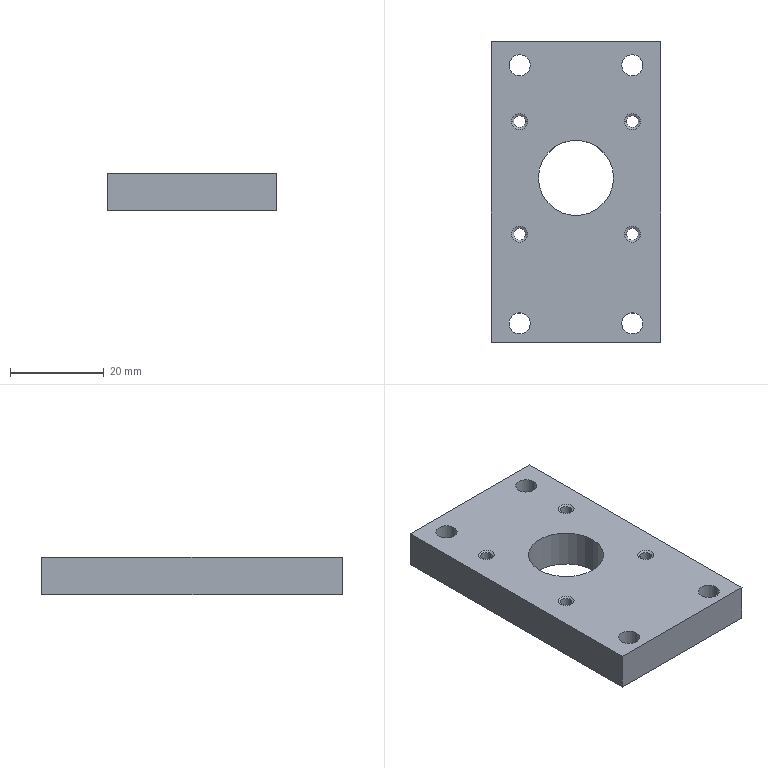Part | NX | 1 solid | 32 faces | box 36.002 x 64 x 8.011 mm | volume 16155 mm3 | cylinder 18 | cone 8 | plane 6 | commonest cylinder face diameters 2.5 x8 4.5 x8 16 x2
STEP:
#1=CARTESIAN_POINT('',(1234.583,117.5,67.602));
#2=VERTEX_POINT('',#1);
#3=CARTESIAN_POINT('',(1198.583,117.5,67.613));
#4=VERTEX_POINT('',#3);
#5=CARTESIAN_POINT('',(1211.755,117.5,67.609));
#6=DIRECTION('',(-1.,0.,0.0003046));
#7=VECTOR('',#6,1000.);
#8=LINE('',#5,#7);
#9=EDGE_CURVE('',#2,#4,#8,.T.);
#10=ORIENTED_EDGE('',*,*,#9,.F.);
#11=CARTESIAN_POINT('',(1234.585,117.5,75.602));
#12=VERTEX_POINT('',#11);
#13=CARTESIAN_POINT('',(1234.582,117.5,65.602));
#14=DIRECTION('',(0.0003046,0.,1.));
#15=VECTOR('',#14,1000.);
#16=LINE('',#13,#15);
#17=EDGE_CURVE('',#2,#12,#16,.T.);
#18=ORIENTED_EDGE('',*,*,#17,.T.);
#19=CARTESIAN_POINT('',(1198.585,117.5,75.613));
#20=VERTEX_POINT('',#19);
#21=CARTESIAN_POINT('',(1211.758,117.5,75.609));
#22=DIRECTION('',(-1.,0.,0.0003046));
#23=VECTOR('',#22,1000.);
#24=LINE('',#21,#23);
#25=EDGE_CURVE('',#12,#20,#24,.T.);
#26=ORIENTED_EDGE('',*,*,#25,.T.);
#27=CARTESIAN_POINT('',(1198.582,117.5,65.613));
#28=DIRECTION('',(-0.0003046,0.,-1.));
#29=VECTOR('',#28,1000.);
#30=LINE('',#27,#29);
#31=EDGE_CURVE('',#20,#4,#30,.T.);
#32=ORIENTED_EDGE('',*,*,#31,.T.);
#33=EDGE_LOOP('',(#10,#18,#26,#32));
#34=FACE_BOUND('',#33,.T.);
#35=CARTESIAN_POINT('',(1236.582,117.5,65.601));
#36=DIRECTION('',(0.,-1.,0.));
#37=DIRECTION('',(0.,0.,-1.));
#38=AXIS2_PLACEMENT_3D('',#35,#36,#37);
#39=PLANE('',#38);
#40=ADVANCED_FACE('',(#34),#39,.T.);
#41=CARTESIAN_POINT('',(1234.583,181.5,67.602));
#42=VERTEX_POINT('',#41);
#43=CARTESIAN_POINT('',(1234.583,131.898,67.602));
#44=DIRECTION('',(0.,-1.,0.));
#45=VECTOR('',#44,1000.);
#46=LINE('',#43,#45);
#47=EDGE_CURVE('',#42,#2,#46,.T.);
#48=ORIENTED_EDGE('',*,*,#47,.F.);
#49=CARTESIAN_POINT('',(1234.585,181.5,75.602));
#50=VERTEX_POINT('',#49);
#51=CARTESIAN_POINT('',(1234.582,181.5,65.602));
#52=DIRECTION('',(0.0003046,0.,1.));
#53=VECTOR('',#52,1000.);
#54=LINE('',#51,#53);
#55=EDGE_CURVE('',#42,#50,#54,.T.);
#56=ORIENTED_EDGE('',*,*,#55,.T.);
#57=CARTESIAN_POINT('',(1234.585,131.898,75.602));
#58=DIRECTION('',(0.,-1.,0.));
#59=VECTOR('',#58,1000.);
#60=LINE('',#57,#59);
#61=EDGE_CURVE('',#50,#12,#60,.T.);
#62=ORIENTED_EDGE('',*,*,#61,.T.);
#63=ORIENTED_EDGE('',*,*,#17,.F.);
#64=EDGE_LOOP('',(#48,#56,#62,#63));
#65=FACE_BOUND('',#64,.T.);
#66=CARTESIAN_POINT('',(1234.582,127.5,65.602));
#67=DIRECTION('',(1.,0.,-0.0003046));
#68=DIRECTION('',(0.,-1.,0.));
#69=AXIS2_PLACEMENT_3D('',#66,#67,#68);
#70=PLANE('',#69);
#71=ADVANCED_FACE('',(#65),#70,.T.);
#72=CARTESIAN_POINT('',(1198.583,181.5,67.613));
#73=VERTEX_POINT('',#72);
#74=CARTESIAN_POINT('',(1211.755,181.5,67.609));
#75=DIRECTION('',(1.,0.,-0.0003046));
#76=VECTOR('',#75,1000.);
#77=LINE('',#74,#76);
#78=EDGE_CURVE('',#73,#42,#77,.T.);
#79=ORIENTED_EDGE('',*,*,#78,.F.);
#80=CARTESIAN_POINT('',(1198.585,181.5,75.613));
#81=VERTEX_POINT('',#80);
#82=CARTESIAN_POINT('',(1198.582,181.5,65.613));
#83=DIRECTION('',(-0.0003046,0.,-1.));
#84=VECTOR('',#83,1000.);
#85=LINE('',#82,#84);
#86=EDGE_CURVE('',#81,#73,#85,.T.);
#87=ORIENTED_EDGE('',*,*,#86,.F.);
#88=CARTESIAN_POINT('',(1211.758,181.5,75.609));
#89=DIRECTION('',(1.,0.,-0.0003046));
#90=VECTOR('',#89,1000.);
#91=LINE('',#88,#90);
#92=EDGE_CURVE('',#81,#50,#91,.T.);
#93=ORIENTED_EDGE('',*,*,#92,.T.);
#94=ORIENTED_EDGE('',*,*,#55,.F.);
#95=EDGE_LOOP('',(#79,#87,#93,#94));
#96=FACE_BOUND('',#95,.T.);
#97=CARTESIAN_POINT('',(1196.582,181.5,65.614));
#98=DIRECTION('',(0.,1.,0.));
#99=DIRECTION('',(0.,0.,-1.));
#100=AXIS2_PLACEMENT_3D('',#97,#98,#99);
#101=PLANE('',#100);
#102=ADVANCED_FACE('',(#96),#101,.T.);
#103=CARTESIAN_POINT('',(1198.583,131.898,67.613));
#104=DIRECTION('',(0.,1.,0.));
#105=VECTOR('',#104,1000.);
#106=LINE('',#103,#105);
#107=EDGE_CURVE('',#4,#73,#106,.T.);
#108=ORIENTED_EDGE('',*,*,#107,.F.);
#109=ORIENTED_EDGE('',*,*,#31,.F.);
#110=CARTESIAN_POINT('',(1198.585,131.898,75.613));
#111=DIRECTION('',(0.,1.,0.));
#112=VECTOR('',#111,1000.);
#113=LINE('',#110,#112);
#114=EDGE_CURVE('',#20,#81,#113,.T.);
#115=ORIENTED_EDGE('',*,*,#114,.T.);
#116=ORIENTED_EDGE('',*,*,#86,.T.);
#117=EDGE_LOOP('',(#108,#109,#115,#116));
#118=FACE_BOUND('',#117,.T.);
#119=CARTESIAN_POINT('',(1198.582,117.5,65.613));
#120=DIRECTION('',(-1.,0.,0.0003046));
#121=DIRECTION('',(0.,1.,0.));
#122=AXIS2_PLACEMENT_3D('',#119,#120,#121);
#123=PLANE('',#122);
#124=ADVANCED_FACE('',(#118),#123,.T.);
#125=ORIENTED_EDGE('',*,*,#61,.F.);
#126=ORIENTED_EDGE('',*,*,#92,.F.);
#127=ORIENTED_EDGE('',*,*,#114,.F.);
#128=ORIENTED_EDGE('',*,*,#25,.F.);
#129=EDGE_LOOP('',(#125,#126,#127,#128));
#130=FACE_BOUND('',#129,.T.);
#131=CARTESIAN_POINT('',(1208.585,152.5,75.61));
#132=VERTEX_POINT('',#131);
#133=CARTESIAN_POINT('',(1224.585,152.5,75.605));
#134=VERTEX_POINT('',#133);
#135=CARTESIAN_POINT('',(1216.585,152.5,75.608));
#136=DIRECTION('',(-0.0003046,0.,-1.));
#137=DIRECTION('',(-1.,0.,0.0003046));
#138=AXIS2_PLACEMENT_3D('',#135,#136,#137);
#139=CIRCLE('',#138,8.);
#140=EDGE_CURVE('',#132,#134,#139,.T.);
#141=ORIENTED_EDGE('',*,*,#140,.T.);
#142=CARTESIAN_POINT('',(1216.585,152.5,75.608));
#143=DIRECTION('',(-0.0003046,0.,-1.));
#144=DIRECTION('',(-1.,0.,0.0003046));
#145=AXIS2_PLACEMENT_3D('',#142,#143,#144);
#146=CIRCLE('',#145,8.);
#147=EDGE_CURVE('',#134,#132,#146,.T.);
#148=ORIENTED_EDGE('',*,*,#147,.T.);
#149=EDGE_LOOP('',(#141,#148));
#150=FACE_BOUND('',#149,.T.);
#151=CARTESIAN_POINT('',(1206.285,140.5,75.611));
#152=VERTEX_POINT('',#151);
#153=CARTESIAN_POINT('',(1202.885,140.5,75.612));
#154=VERTEX_POINT('',#153);
#155=CARTESIAN_POINT('',(1204.585,140.5,75.611));
#156=DIRECTION('',(0.0003046,0.,1.));
#157=DIRECTION('',(1.,0.,-0.0003046));
#158=AXIS2_PLACEMENT_3D('',#155,#156,#157);
#159=CIRCLE('',#158,1.7);
#160=EDGE_CURVE('',#152,#154,#159,.T.);
#161=ORIENTED_EDGE('',*,*,#160,.F.);
#162=CARTESIAN_POINT('',(1204.585,140.5,75.611));
#163=DIRECTION('',(0.0003046,0.,1.));
#164=DIRECTION('',(1.,0.,-0.0003046));
#165=AXIS2_PLACEMENT_3D('',#162,#163,#164);
#166=CIRCLE('',#165,1.7);
#167=EDGE_CURVE('',#154,#152,#166,.T.);
#168=ORIENTED_EDGE('',*,*,#167,.F.);
#169=EDGE_LOOP('',(#161,#168));
#170=FACE_BOUND('',#169,.T.);
#171=CARTESIAN_POINT('',(1202.885,164.5,75.612));
#172=VERTEX_POINT('',#171);
#173=CARTESIAN_POINT('',(1206.285,164.5,75.611));
#174=VERTEX_POINT('',#173);
#175=CARTESIAN_POINT('',(1204.585,164.5,75.611));
#176=DIRECTION('',(0.0003046,0.,1.));
#177=DIRECTION('',(1.,0.,-0.0003046));
#178=AXIS2_PLACEMENT_3D('',#175,#176,#177);
#179=CIRCLE('',#178,1.7);
#180=EDGE_CURVE('',#172,#174,#179,.T.);
#181=ORIENTED_EDGE('',*,*,#180,.F.);
#182=CARTESIAN_POINT('',(1204.585,164.5,75.611));
#183=DIRECTION('',(0.0003046,0.,1.));
#184=DIRECTION('',(1.,0.,-0.0003046));
#185=AXIS2_PLACEMENT_3D('',#182,#183,#184);
#186=CIRCLE('',#185,1.7);
#187=EDGE_CURVE('',#174,#172,#186,.T.);
#188=ORIENTED_EDGE('',*,*,#187,.F.);
#189=EDGE_LOOP('',(#181,#188));
#190=FACE_BOUND('',#189,.T.);
#191=CARTESIAN_POINT('',(1230.835,121.5,75.603));
#192=VERTEX_POINT('',#191);
#193=CARTESIAN_POINT('',(1226.335,121.5,75.605));
#194=VERTEX_POINT('',#193);
#195=CARTESIAN_POINT('',(1228.585,121.5,75.604));
#196=DIRECTION('',(0.0003046,0.,1.));
#197=DIRECTION('',(1.,0.,-0.0003046));
#198=AXIS2_PLACEMENT_3D('',#195,#196,#197);
#199=CIRCLE('',#198,2.25);
#200=EDGE_CURVE('',#192,#194,#199,.T.);
#201=ORIENTED_EDGE('',*,*,#200,.F.);
#202=CARTESIAN_POINT('',(1228.585,121.5,75.604));
#203=DIRECTION('',(0.0003046,0.,1.));
#204=DIRECTION('',(1.,0.,-0.0003046));
#205=AXIS2_PLACEMENT_3D('',#202,#203,#204);
#206=CIRCLE('',#205,2.25);
#207=EDGE_CURVE('',#194,#192,#206,.T.);
#208=ORIENTED_EDGE('',*,*,#207,.F.);
#209=EDGE_LOOP('',(#201,#208));
#210=FACE_BOUND('',#209,.T.);
#211=CARTESIAN_POINT('',(1202.335,121.5,75.612));
#212=VERTEX_POINT('',#211);
#213=CARTESIAN_POINT('',(1206.835,121.5,75.611));
#214=VERTEX_POINT('',#213);
#215=CARTESIAN_POINT('',(1204.585,121.5,75.611));
#216=DIRECTION('',(0.0003046,0.,1.));
#217=DIRECTION('',(1.,0.,-0.0003046));
#218=AXIS2_PLACEMENT_3D('',#215,#216,#217);
#219=CIRCLE('',#218,2.25);
#220=EDGE_CURVE('',#212,#214,#219,.T.);
#221=ORIENTED_EDGE('',*,*,#220,.F.);
#222=CARTESIAN_POINT('',(1204.585,121.5,75.611));
#223=DIRECTION('',(0.0003046,0.,1.));
#224=DIRECTION('',(1.,0.,-0.0003046));
#225=AXIS2_PLACEMENT_3D('',#222,#223,#224);
#226=CIRCLE('',#225,2.25);
#227=EDGE_CURVE('',#214,#212,#226,.T.);
#228=ORIENTED_EDGE('',*,*,#227,.F.);
#229=EDGE_LOOP('',(#221,#228));
#230=FACE_BOUND('',#229,.T.);
#231=CARTESIAN_POINT('',(1202.335,176.5,75.612));
#232=VERTEX_POINT('',#231);
#233=CARTESIAN_POINT('',(1206.835,176.5,75.611));
#234=VERTEX_POINT('',#233);
#235=CARTESIAN_POINT('',(1204.585,176.5,75.611));
#236=DIRECTION('',(0.0003046,0.,1.));
#237=DIRECTION('',(1.,0.,-0.0003046));
#238=AXIS2_PLACEMENT_3D('',#235,#236,#237);
#239=CIRCLE('',#238,2.25);
#240=EDGE_CURVE('',#232,#234,#239,.T.);
#241=ORIENTED_EDGE('',*,*,#240,.F.);
#242=CARTESIAN_POINT('',(1204.585,176.5,75.611));
#243=DIRECTION('',(0.0003046,0.,1.));
#244=DIRECTION('',(1.,0.,-0.0003046));
#245=AXIS2_PLACEMENT_3D('',#242,#243,#244);
#246=CIRCLE('',#245,2.25);
#247=EDGE_CURVE('',#234,#232,#246,.T.);
#248=ORIENTED_EDGE('',*,*,#247,.F.);
#249=EDGE_LOOP('',(#241,#248));
#250=FACE_BOUND('',#249,.T.);
#251=CARTESIAN_POINT('',(1230.835,176.5,75.603));
#252=VERTEX_POINT('',#251);
#253=CARTESIAN_POINT('',(1226.335,176.5,75.605));
#254=VERTEX_POINT('',#253);
#255=CARTESIAN_POINT('',(1228.585,176.5,75.604));
#256=DIRECTION('',(0.0003046,0.,1.));
#257=DIRECTION('',(1.,0.,-0.0003046));
#258=AXIS2_PLACEMENT_3D('',#255,#256,#257);
#259=CIRCLE('',#258,2.25);
#260=EDGE_CURVE('',#252,#254,#259,.T.);
#261=ORIENTED_EDGE('',*,*,#260,.F.);
#262=CARTESIAN_POINT('',(1228.585,176.5,75.604));
#263=DIRECTION('',(0.0003046,0.,1.));
#264=DIRECTION('',(1.,0.,-0.0003046));
#265=AXIS2_PLACEMENT_3D('',#262,#263,#264);
#266=CIRCLE('',#265,2.25);
#267=EDGE_CURVE('',#254,#252,#266,.T.);
#268=ORIENTED_EDGE('',*,*,#267,.F.);
#269=EDGE_LOOP('',(#261,#268));
#270=FACE_BOUND('',#269,.T.);
#271=CARTESIAN_POINT('',(1226.885,164.5,75.604));
#272=VERTEX_POINT('',#271);
#273=CARTESIAN_POINT('',(1230.285,164.5,75.603));
#274=VERTEX_POINT('',#273);
#275=CARTESIAN_POINT('',(1228.585,164.5,75.604));
#276=DIRECTION('',(0.0003046,0.,1.));
#277=DIRECTION('',(1.,0.,-0.0003046));
#278=AXIS2_PLACEMENT_3D('',#275,#276,#277);
#279=CIRCLE('',#278,1.7);
#280=EDGE_CURVE('',#272,#274,#279,.T.);
#281=ORIENTED_EDGE('',*,*,#280,.F.);
#282=CARTESIAN_POINT('',(1228.585,164.5,75.604));
#283=DIRECTION('',(0.0003046,0.,1.));
#284=DIRECTION('',(1.,0.,-0.0003046));
#285=AXIS2_PLACEMENT_3D('',#282,#283,#284);
#286=CIRCLE('',#285,1.7);
#287=EDGE_CURVE('',#274,#272,#286,.T.);
#288=ORIENTED_EDGE('',*,*,#287,.F.);
#289=EDGE_LOOP('',(#281,#288));
#290=FACE_BOUND('',#289,.T.);
#291=CARTESIAN_POINT('',(1226.885,140.5,75.604));
#292=VERTEX_POINT('',#291);
#293=CARTESIAN_POINT('',(1230.285,140.5,75.603));
#294=VERTEX_POINT('',#293);
#295=CARTESIAN_POINT('',(1228.585,140.5,75.604));
#296=DIRECTION('',(0.0003046,0.,1.));
#297=DIRECTION('',(1.,0.,-0.0003046));
#298=AXIS2_PLACEMENT_3D('',#295,#296,#297);
#299=CIRCLE('',#298,1.7);
#300=EDGE_CURVE('',#292,#294,#299,.T.);
#301=ORIENTED_EDGE('',*,*,#300,.F.);
#302=CARTESIAN_POINT('',(1228.585,140.5,75.604));
#303=DIRECTION('',(0.0003046,0.,1.));
#304=DIRECTION('',(1.,0.,-0.0003046));
#305=AXIS2_PLACEMENT_3D('',#302,#303,#304);
#306=CIRCLE('',#305,1.7);
#307=EDGE_CURVE('',#294,#292,#306,.T.);
#308=ORIENTED_EDGE('',*,*,#307,.F.);
#309=EDGE_LOOP('',(#301,#308));
#310=FACE_BOUND('',#309,.T.);
#311=CARTESIAN_POINT('',(1211.758,131.898,75.609));
#312=DIRECTION('',(0.0003046,0.,1.));
#313=DIRECTION('',(-0.000000134,-1.,0.));
#314=AXIS2_PLACEMENT_3D('',#311,#312,#313);
#315=PLANE('',#314);
#316=ADVANCED_FACE('',(#130,#150,#170,#190,#210,#230,#250,#270,#290,#310),#315,.T.);
#317=ORIENTED_EDGE('',*,*,#140,.F.);
#318=CARTESIAN_POINT('',(1208.583,152.5,67.61));
#319=VERTEX_POINT('',#318);
#320=CARTESIAN_POINT('',(1208.585,152.5,76.625));
#321=DIRECTION('',(-0.0003046,0.,-1.));
#322=VECTOR('',#321,1000.);
#323=LINE('',#320,#322);
#324=EDGE_CURVE('',#319,#132,#323,.F.);
#325=ORIENTED_EDGE('',*,*,#324,.F.);
#326=CARTESIAN_POINT('',(1224.583,152.5,67.605));
#327=VERTEX_POINT('',#326);
#328=CARTESIAN_POINT('',(1216.583,152.5,67.608));
#329=DIRECTION('',(-0.0003046,0.,-1.));
#330=DIRECTION('',(-1.,0.,0.0003046));
#331=AXIS2_PLACEMENT_3D('',#328,#329,#330);
#332=CIRCLE('',#331,8.);
#333=EDGE_CURVE('',#319,#327,#332,.T.);
#334=ORIENTED_EDGE('',*,*,#333,.T.);
#335=CARTESIAN_POINT('',(1224.585,152.5,76.62));
#336=DIRECTION('',(-0.0003046,0.,-1.));
#337=VECTOR('',#336,1000.);
#338=LINE('',#335,#337);
#339=EDGE_CURVE('',#327,#134,#338,.F.);
#340=ORIENTED_EDGE('',*,*,#339,.T.);
#341=EDGE_LOOP('',(#317,#325,#334,#340));
#342=FACE_BOUND('',#341,.T.);
#343=CARTESIAN_POINT('',(1216.585,152.5,76.622));
#344=DIRECTION('',(-0.0003046,0.,-1.));
#345=DIRECTION('',(-1.,0.,0.0003046));
#346=AXIS2_PLACEMENT_3D('',#343,#344,#345);
#347=CYLINDRICAL_SURFACE('',#346,8.);
#348=ADVANCED_FACE('',(#342),#347,.F.);
#349=ORIENTED_EDGE('',*,*,#240,.T.);
#350=CARTESIAN_POINT('',(1206.833,176.5,67.611));
#351=VERTEX_POINT('',#350);
#352=CARTESIAN_POINT('',(1206.832,176.5,66.797));
#353=DIRECTION('',(0.0003046,0.,1.));
#354=VECTOR('',#353,1000.);
#355=LINE('',#352,#354);
#356=EDGE_CURVE('',#351,#234,#355,.T.);
#357=ORIENTED_EDGE('',*,*,#356,.F.);
#358=CARTESIAN_POINT('',(1202.333,176.5,67.612));
#359=VERTEX_POINT('',#358);
#360=CARTESIAN_POINT('',(1204.583,176.5,67.611));
#361=DIRECTION('',(0.0003046,0.,1.));
#362=DIRECTION('',(1.,0.,-0.0003046));
#363=AXIS2_PLACEMENT_3D('',#360,#361,#362);
#364=CIRCLE('',#363,2.25);
#365=EDGE_CURVE('',#359,#351,#364,.T.);
#366=ORIENTED_EDGE('',*,*,#365,.F.);
#367=CARTESIAN_POINT('',(1202.332,176.5,66.799));
#368=DIRECTION('',(0.0003046,0.,1.));
#369=VECTOR('',#368,1000.);
#370=LINE('',#367,#369);
#371=EDGE_CURVE('',#359,#232,#370,.T.);
#372=ORIENTED_EDGE('',*,*,#371,.T.);
#373=EDGE_LOOP('',(#349,#357,#366,#372));
#374=FACE_BOUND('',#373,.T.);
#375=CARTESIAN_POINT('',(1204.582,176.5,66.798));
#376=DIRECTION('',(0.0003046,0.,1.));
#377=DIRECTION('',(1.,0.,-0.0003046));
#378=AXIS2_PLACEMENT_3D('',#375,#376,#377);
#379=CYLINDRICAL_SURFACE('',#378,2.25);
#380=ADVANCED_FACE('',(#374),#379,.F.);
#381=CARTESIAN_POINT('',(1230.833,176.5,67.603));
#382=VERTEX_POINT('',#381);
#383=CARTESIAN_POINT('',(1226.333,176.5,67.605));
#384=VERTEX_POINT('',#383);
#385=CARTESIAN_POINT('',(1228.583,176.5,67.604));
#386=DIRECTION('',(0.0003046,0.,1.));
#387=DIRECTION('',(1.,0.,-0.0003046));
#388=AXIS2_PLACEMENT_3D('',#385,#386,#387);
#389=CIRCLE('',#388,2.25);
#390=EDGE_CURVE('',#382,#384,#389,.T.);
#391=ORIENTED_EDGE('',*,*,#390,.F.);
#392=CARTESIAN_POINT('',(1230.832,176.5,66.79));
#393=DIRECTION('',(0.0003046,0.,1.));
#394=VECTOR('',#393,1000.);
#395=LINE('',#392,#394);
#396=EDGE_CURVE('',#382,#252,#395,.T.);
#397=ORIENTED_EDGE('',*,*,#396,.T.);
#398=ORIENTED_EDGE('',*,*,#260,.T.);
#399=CARTESIAN_POINT('',(1226.332,176.5,66.791));
#400=DIRECTION('',(0.0003046,0.,1.));
#401=VECTOR('',#400,1000.);
#402=LINE('',#399,#401);
#403=EDGE_CURVE('',#384,#254,#402,.T.);
#404=ORIENTED_EDGE('',*,*,#403,.F.);
#405=EDGE_LOOP('',(#391,#397,#398,#404));
#406=FACE_BOUND('',#405,.T.);
#407=CARTESIAN_POINT('',(1228.582,176.5,66.791));
#408=DIRECTION('',(0.0003046,0.,1.));
#409=DIRECTION('',(1.,0.,-0.0003046));
#410=AXIS2_PLACEMENT_3D('',#407,#408,#409);
#411=CYLINDRICAL_SURFACE('',#410,2.25);
#412=ADVANCED_FACE('',(#406),#411,.F.);
#413=ORIENTED_EDGE('',*,*,#220,.T.);
#414=CARTESIAN_POINT('',(1206.833,121.5,67.611));
#415=VERTEX_POINT('',#414);
#416=CARTESIAN_POINT('',(1206.832,121.5,64.596));
#417=DIRECTION('',(0.0003046,0.,1.));
#418=VECTOR('',#417,1000.);
#419=LINE('',#416,#418);
#420=EDGE_CURVE('',#415,#214,#419,.T.);
#421=ORIENTED_EDGE('',*,*,#420,.F.);
#422=CARTESIAN_POINT('',(1202.333,121.5,67.612));
#423=VERTEX_POINT('',#422);
#424=CARTESIAN_POINT('',(1204.583,121.5,67.611));
#425=DIRECTION('',(0.0003046,0.,1.));
#426=DIRECTION('',(1.,0.,-0.0003046));
#427=AXIS2_PLACEMENT_3D('',#424,#425,#426);
#428=CIRCLE('',#427,2.25);
#429=EDGE_CURVE('',#423,#415,#428,.T.);
#430=ORIENTED_EDGE('',*,*,#429,.F.);
#431=CARTESIAN_POINT('',(1202.332,121.5,64.597));
#432=DIRECTION('',(0.0003046,0.,1.));
#433=VECTOR('',#432,1000.);
#434=LINE('',#431,#433);
#435=EDGE_CURVE('',#423,#212,#434,.T.);
#436=ORIENTED_EDGE('',*,*,#435,.T.);
#437=EDGE_LOOP('',(#413,#421,#430,#436));
#438=FACE_BOUND('',#437,.T.);
#439=CARTESIAN_POINT('',(1204.582,121.5,64.597));
#440=DIRECTION('',(0.0003046,0.,1.));
#441=DIRECTION('',(1.,0.,-0.0003046));
#442=AXIS2_PLACEMENT_3D('',#439,#440,#441);
#443=CYLINDRICAL_SURFACE('',#442,2.25);
#444=ADVANCED_FACE('',(#438),#443,.F.);
#445=CARTESIAN_POINT('',(1230.833,121.5,67.603));
#446=VERTEX_POINT('',#445);
#447=CARTESIAN_POINT('',(1226.333,121.5,67.605));
#448=VERTEX_POINT('',#447);
#449=CARTESIAN_POINT('',(1228.583,121.5,67.604));
#450=DIRECTION('',(0.0003046,0.,1.));
#451=DIRECTION('',(1.,0.,-0.0003046));
#452=AXIS2_PLACEMENT_3D('',#449,#450,#451);
#453=CIRCLE('',#452,2.25);
#454=EDGE_CURVE('',#446,#448,#453,.T.);
#455=ORIENTED_EDGE('',*,*,#454,.F.);
#456=CARTESIAN_POINT('',(1230.832,121.5,64.589));
#457=DIRECTION('',(0.0003046,0.,1.));
#458=VECTOR('',#457,1000.);
#459=LINE('',#456,#458);
#460=EDGE_CURVE('',#446,#192,#459,.T.);
#461=ORIENTED_EDGE('',*,*,#460,.T.);
#462=ORIENTED_EDGE('',*,*,#200,.T.);
#463=CARTESIAN_POINT('',(1226.332,121.5,64.59));
#464=DIRECTION('',(0.0003046,0.,1.));
#465=VECTOR('',#464,1000.);
#466=LINE('',#463,#465);
#467=EDGE_CURVE('',#448,#194,#466,.T.);
#468=ORIENTED_EDGE('',*,*,#467,.F.);
#469=EDGE_LOOP('',(#455,#461,#462,#468));
#470=FACE_BOUND('',#469,.T.);
#471=CARTESIAN_POINT('',(1228.582,121.5,64.589));
#472=DIRECTION('',(0.0003046,0.,1.));
#473=DIRECTION('',(1.,0.,-0.0003046));
#474=AXIS2_PLACEMENT_3D('',#471,#472,#473);
#475=CYLINDRICAL_SURFACE('',#474,2.25);
#476=ADVANCED_FACE('',(#470),#475,.F.);
#477=CARTESIAN_POINT('',(1227.333,164.5,67.604));
#478=VERTEX_POINT('',#477);
#479=CARTESIAN_POINT('',(1229.833,164.5,67.604));
#480=VERTEX_POINT('',#479);
#481=CARTESIAN_POINT('',(1228.583,164.5,67.604));
#482=DIRECTION('',(0.0003046,0.,1.));
#483=DIRECTION('',(1.,0.,-0.0003046));
#484=AXIS2_PLACEMENT_3D('',#481,#482,#483);
#485=CIRCLE('',#484,1.25);
#486=EDGE_CURVE('',#478,#480,#485,.T.);
#487=ORIENTED_EDGE('',*,*,#486,.F.);
#488=CARTESIAN_POINT('',(1227.335,164.5,75.344));
#489=VERTEX_POINT('',#488);
#490=CARTESIAN_POINT('',(1227.335,164.5,75.604));
#491=DIRECTION('',(0.0003046,0.,1.));
#492=VECTOR('',#491,1000.);
#493=LINE('',#490,#492);
#494=EDGE_CURVE('',#489,#478,#493,.F.);
#495=ORIENTED_EDGE('',*,*,#494,.F.);
#496=CARTESIAN_POINT('',(1229.835,164.5,75.344));
#497=VERTEX_POINT('',#496);
#498=CARTESIAN_POINT('',(1228.585,164.5,75.344));
#499=DIRECTION('',(0.0003046,0.,1.));
#500=DIRECTION('',(1.,0.,-0.0003046));
#501=AXIS2_PLACEMENT_3D('',#498,#499,#500);
#502=CIRCLE('',#501,1.25);
#503=EDGE_CURVE('',#489,#497,#502,.T.);
#504=ORIENTED_EDGE('',*,*,#503,.T.);
#505=CARTESIAN_POINT('',(1229.835,164.5,75.604));
#506=DIRECTION('',(0.0003046,0.,1.));
#507=VECTOR('',#506,1000.);
#508=LINE('',#505,#507);
#509=EDGE_CURVE('',#497,#480,#508,.F.);
#510=ORIENTED_EDGE('',*,*,#509,.T.);
#511=EDGE_LOOP('',(#487,#495,#504,#510));
#512=FACE_BOUND('',#511,.T.);
#513=CARTESIAN_POINT('',(1228.585,164.5,75.604));
#514=DIRECTION('',(0.0003046,0.,1.));
#515=DIRECTION('',(1.,0.,-0.0003046));
#516=AXIS2_PLACEMENT_3D('',#513,#514,#515);
#517=CYLINDRICAL_SURFACE('',#516,1.25);
#518=ADVANCED_FACE('',(#512),#517,.F.);
#519=CARTESIAN_POINT('',(1228.585,164.5,75.344));
#520=DIRECTION('',(0.0003046,0.,1.));
#521=DIRECTION('',(1.,0.,-0.0003046));
#522=AXIS2_PLACEMENT_3D('',#519,#520,#521);
#523=CIRCLE('',#522,1.25);
#524=EDGE_CURVE('',#497,#489,#523,.T.);
#525=ORIENTED_EDGE('',*,*,#524,.F.);
#526=CARTESIAN_POINT('',(1229.835,164.5,75.344));
#527=DIRECTION('',(0.8662,0.,0.4997));
#528=VECTOR('',#527,1000.);
#529=LINE('',#526,#528);
#530=EDGE_CURVE('',#497,#274,#529,.T.);
#531=ORIENTED_EDGE('',*,*,#530,.T.);
#532=ORIENTED_EDGE('',*,*,#287,.T.);
#533=CARTESIAN_POINT('',(1227.335,164.5,75.344));
#534=DIRECTION('',(-0.8659,0.,0.5003));
#535=VECTOR('',#534,1000.);
#536=LINE('',#533,#535);
#537=EDGE_CURVE('',#489,#272,#536,.T.);
#538=ORIENTED_EDGE('',*,*,#537,.F.);
#539=EDGE_LOOP('',(#525,#531,#532,#538));
#540=FACE_BOUND('',#539,.T.);
#541=CARTESIAN_POINT('',(1228.585,164.5,75.344));
#542=DIRECTION('',(0.0003046,0.,1.));
#543=DIRECTION('',(1.,0.,-0.0003046));
#544=AXIS2_PLACEMENT_3D('',#541,#542,#543);
#545=CONICAL_SURFACE('',#544,1.25,1.047);
#546=ADVANCED_FACE('',(#540),#545,.F.);
#547=CARTESIAN_POINT('',(1205.835,164.5,75.351));
#548=VERTEX_POINT('',#547);
#549=CARTESIAN_POINT('',(1203.335,164.5,75.352));
#550=VERTEX_POINT('',#549);
#551=CARTESIAN_POINT('',(1204.585,164.5,75.351));
#552=DIRECTION('',(0.0003046,0.,1.));
#553=DIRECTION('',(1.,0.,-0.0003046));
#554=AXIS2_PLACEMENT_3D('',#551,#552,#553);
#555=CIRCLE('',#554,1.25);
#556=EDGE_CURVE('',#548,#550,#555,.T.);
#557=ORIENTED_EDGE('',*,*,#556,.T.);
#558=CARTESIAN_POINT('',(1203.333,164.5,67.612));
#559=VERTEX_POINT('',#558);
#560=CARTESIAN_POINT('',(1203.335,164.5,75.612));
#561=DIRECTION('',(0.0003046,0.,1.));
#562=VECTOR('',#561,1000.);
#563=LINE('',#560,#562);
#564=EDGE_CURVE('',#550,#559,#563,.F.);
#565=ORIENTED_EDGE('',*,*,#564,.T.);
#566=CARTESIAN_POINT('',(1205.833,164.5,67.611));
#567=VERTEX_POINT('',#566);
#568=CARTESIAN_POINT('',(1204.583,164.5,67.611));
#569=DIRECTION('',(0.0003046,0.,1.));
#570=DIRECTION('',(1.,0.,-0.0003046));
#571=AXIS2_PLACEMENT_3D('',#568,#569,#570);
#572=CIRCLE('',#571,1.25);
#573=EDGE_CURVE('',#567,#559,#572,.T.);
#574=ORIENTED_EDGE('',*,*,#573,.F.);
#575=CARTESIAN_POINT('',(1205.835,164.5,75.611));
#576=DIRECTION('',(0.0003046,0.,1.));
#577=VECTOR('',#576,1000.);
#578=LINE('',#575,#577);
#579=EDGE_CURVE('',#548,#567,#578,.F.);
#580=ORIENTED_EDGE('',*,*,#579,.F.);
#581=EDGE_LOOP('',(#557,#565,#574,#580));
#582=FACE_BOUND('',#581,.T.);
#583=CARTESIAN_POINT('',(1204.585,164.5,75.611));
#584=DIRECTION('',(0.0003046,0.,1.));
#585=DIRECTION('',(1.,0.,-0.0003046));
#586=AXIS2_PLACEMENT_3D('',#583,#584,#585);
#587=CYLINDRICAL_SURFACE('',#586,1.25);
#588=ADVANCED_FACE('',(#582),#587,.F.);
#589=ORIENTED_EDGE('',*,*,#556,.F.);
#590=CARTESIAN_POINT('',(1205.835,164.5,75.351));
#591=DIRECTION('',(0.8662,0.,0.4997));
#592=VECTOR('',#591,1000.);
#593=LINE('',#590,#592);
#594=EDGE_CURVE('',#548,#174,#593,.T.);
#595=ORIENTED_EDGE('',*,*,#594,.T.);
#596=ORIENTED_EDGE('',*,*,#187,.T.);
#597=CARTESIAN_POINT('',(1203.335,164.5,75.352));
#598=DIRECTION('',(-0.8659,0.,0.5003));
#599=VECTOR('',#598,1000.);
#600=LINE('',#597,#599);
#601=EDGE_CURVE('',#550,#172,#600,.T.);
#602=ORIENTED_EDGE('',*,*,#601,.F.);
#603=EDGE_LOOP('',(#589,#595,#596,#602));
#604=FACE_BOUND('',#603,.T.);
#605=CARTESIAN_POINT('',(1204.585,164.5,75.351));
#606=DIRECTION('',(0.0003046,0.,1.));
#607=DIRECTION('',(1.,0.,-0.0003046));
#608=AXIS2_PLACEMENT_3D('',#605,#606,#607);
#609=CONICAL_SURFACE('',#608,1.25,1.047);
#610=ADVANCED_FACE('',(#604),#609,.F.);
#611=CARTESIAN_POINT('',(1229.833,140.5,67.604));
#612=VERTEX_POINT('',#611);
#613=CARTESIAN_POINT('',(1227.333,140.5,67.604));
#614=VERTEX_POINT('',#613);
#615=CARTESIAN_POINT('',(1228.583,140.5,67.604));
#616=DIRECTION('',(0.0003046,0.,1.));
#617=DIRECTION('',(1.,0.,-0.0003046));
#618=AXIS2_PLACEMENT_3D('',#615,#616,#617);
#619=CIRCLE('',#618,1.25);
#620=EDGE_CURVE('',#612,#614,#619,.T.);
#621=ORIENTED_EDGE('',*,*,#620,.F.);
#622=CARTESIAN_POINT('',(1229.835,140.5,75.344));
#623=VERTEX_POINT('',#622);
#624=CARTESIAN_POINT('',(1229.835,140.5,75.604));
#625=DIRECTION('',(0.0003046,0.,1.));
#626=VECTOR('',#625,1000.);
#627=LINE('',#624,#626);
#628=EDGE_CURVE('',#612,#623,#627,.T.);
#629=ORIENTED_EDGE('',*,*,#628,.T.);
#630=CARTESIAN_POINT('',(1227.335,140.5,75.344));
#631=VERTEX_POINT('',#630);
#632=CARTESIAN_POINT('',(1228.585,140.5,75.344));
#633=DIRECTION('',(0.0003046,0.,1.));
#634=DIRECTION('',(1.,0.,-0.0003046));
#635=AXIS2_PLACEMENT_3D('',#632,#633,#634);
#636=CIRCLE('',#635,1.25);
#637=EDGE_CURVE('',#623,#631,#636,.T.);
#638=ORIENTED_EDGE('',*,*,#637,.T.);
#639=CARTESIAN_POINT('',(1227.335,140.5,75.604));
#640=DIRECTION('',(0.0003046,0.,1.));
#641=VECTOR('',#640,1000.);
#642=LINE('',#639,#641);
#643=EDGE_CURVE('',#614,#631,#642,.T.);
#644=ORIENTED_EDGE('',*,*,#643,.F.);
#645=EDGE_LOOP('',(#621,#629,#638,#644));
#646=FACE_BOUND('',#645,.T.);
#647=CARTESIAN_POINT('',(1228.585,140.5,75.604));
#648=DIRECTION('',(0.0003046,0.,1.));
#649=DIRECTION('',(1.,0.,-0.0003046));
#650=AXIS2_PLACEMENT_3D('',#647,#648,#649);
#651=CYLINDRICAL_SURFACE('',#650,1.25);
#652=ADVANCED_FACE('',(#646),#651,.F.);
#653=CARTESIAN_POINT('',(1228.585,140.5,75.344));
#654=DIRECTION('',(0.0003046,0.,1.));
#655=DIRECTION('',(1.,0.,-0.0003046));
#656=AXIS2_PLACEMENT_3D('',#653,#654,#655);
#657=CIRCLE('',#656,1.25);
#658=EDGE_CURVE('',#631,#623,#657,.T.);
#659=ORIENTED_EDGE('',*,*,#658,.F.);
#660=CARTESIAN_POINT('',(1227.335,140.5,75.344));
#661=DIRECTION('',(-0.8659,0.,0.5003));
#662=VECTOR('',#661,1000.);
#663=LINE('',#660,#662);
#664=EDGE_CURVE('',#631,#292,#663,.T.);
#665=ORIENTED_EDGE('',*,*,#664,.T.);
#666=ORIENTED_EDGE('',*,*,#300,.T.);
#667=CARTESIAN_POINT('',(1229.835,140.5,75.344));
#668=DIRECTION('',(0.8662,0.,0.4997));
#669=VECTOR('',#668,1000.);
#670=LINE('',#667,#669);
#671=EDGE_CURVE('',#623,#294,#670,.T.);
#672=ORIENTED_EDGE('',*,*,#671,.F.);
#673=EDGE_LOOP('',(#659,#665,#666,#672));
#674=FACE_BOUND('',#673,.T.);
#675=CARTESIAN_POINT('',(1228.585,140.5,75.344));
#676=DIRECTION('',(0.0003046,0.,1.));
#677=DIRECTION('',(1.,0.,-0.0003046));
#678=AXIS2_PLACEMENT_3D('',#675,#676,#677);
#679=CONICAL_SURFACE('',#678,1.25,1.047);
#680=ADVANCED_FACE('',(#674),#679,.F.);
#681=CARTESIAN_POINT('',(1205.833,140.5,67.611));
#682=VERTEX_POINT('',#681);
#683=CARTESIAN_POINT('',(1203.333,140.5,67.612));
#684=VERTEX_POINT('',#683);
#685=CARTESIAN_POINT('',(1204.583,140.5,67.611));
#686=DIRECTION('',(0.0003046,0.,1.));
#687=DIRECTION('',(1.,0.,-0.0003046));
#688=AXIS2_PLACEMENT_3D('',#685,#686,#687);
#689=CIRCLE('',#688,1.25);
#690=EDGE_CURVE('',#682,#684,#689,.T.);
#691=ORIENTED_EDGE('',*,*,#690,.F.);
#692=CARTESIAN_POINT('',(1205.835,140.5,75.351));
#693=VERTEX_POINT('',#692);
#694=CARTESIAN_POINT('',(1205.835,140.5,75.611));
#695=DIRECTION('',(0.0003046,0.,1.));
#696=VECTOR('',#695,1000.);
#697=LINE('',#694,#696);
#698=EDGE_CURVE('',#693,#682,#697,.F.);
#699=ORIENTED_EDGE('',*,*,#698,.F.);
#700=CARTESIAN_POINT('',(1203.335,140.5,75.352));
#701=VERTEX_POINT('',#700);
#702=CARTESIAN_POINT('',(1204.585,140.5,75.351));
#703=DIRECTION('',(0.0003046,0.,1.));
#704=DIRECTION('',(1.,0.,-0.0003046));
#705=AXIS2_PLACEMENT_3D('',#702,#703,#704);
#706=CIRCLE('',#705,1.25);
#707=EDGE_CURVE('',#693,#701,#706,.T.);
#708=ORIENTED_EDGE('',*,*,#707,.T.);
#709=CARTESIAN_POINT('',(1203.335,140.5,75.612));
#710=DIRECTION('',(0.0003046,0.,1.));
#711=VECTOR('',#710,1000.);
#712=LINE('',#709,#711);
#713=EDGE_CURVE('',#701,#684,#712,.F.);
#714=ORIENTED_EDGE('',*,*,#713,.T.);
#715=EDGE_LOOP('',(#691,#699,#708,#714));
#716=FACE_BOUND('',#715,.T.);
#717=CARTESIAN_POINT('',(1204.585,140.5,75.611));
#718=DIRECTION('',(0.0003046,0.,1.));
#719=DIRECTION('',(1.,0.,-0.0003046));
#720=AXIS2_PLACEMENT_3D('',#717,#718,#719);
#721=CYLINDRICAL_SURFACE('',#720,1.25);
#722=ADVANCED_FACE('',(#716),#721,.F.);
#723=ORIENTED_EDGE('',*,*,#707,.F.);
#724=CARTESIAN_POINT('',(1205.835,140.5,75.351));
#725=DIRECTION('',(0.8662,0.,0.4997));
#726=VECTOR('',#725,1000.);
#727=LINE('',#724,#726);
#728=EDGE_CURVE('',#693,#152,#727,.T.);
#729=ORIENTED_EDGE('',*,*,#728,.T.);
#730=ORIENTED_EDGE('',*,*,#160,.T.);
#731=CARTESIAN_POINT('',(1203.335,140.5,75.352));
#732=DIRECTION('',(-0.8659,0.,0.5003));
#733=VECTOR('',#732,1000.);
#734=LINE('',#731,#733);
#735=EDGE_CURVE('',#701,#154,#734,.T.);
#736=ORIENTED_EDGE('',*,*,#735,.F.);
#737=EDGE_LOOP('',(#723,#729,#730,#736));
#738=FACE_BOUND('',#737,.T.);
#739=CARTESIAN_POINT('',(1204.585,140.5,75.351));
#740=DIRECTION('',(0.0003046,0.,1.));
#741=DIRECTION('',(1.,0.,-0.0003046));
#742=AXIS2_PLACEMENT_3D('',#739,#740,#741);
#743=CONICAL_SURFACE('',#742,1.25,1.047);
#744=ADVANCED_FACE('',(#738),#743,.F.);
#745=ORIENTED_EDGE('',*,*,#9,.T.);
#746=ORIENTED_EDGE('',*,*,#107,.T.);
#747=ORIENTED_EDGE('',*,*,#78,.T.);
#748=ORIENTED_EDGE('',*,*,#47,.T.);
#749=EDGE_LOOP('',(#745,#746,#747,#748));
#750=FACE_BOUND('',#749,.T.);
#751=CARTESIAN_POINT('',(1216.583,152.5,67.608));
#752=DIRECTION('',(-0.0003046,0.,-1.));
#753=DIRECTION('',(-1.,0.,0.0003046));
#754=AXIS2_PLACEMENT_3D('',#751,#752,#753);
#755=CIRCLE('',#754,8.);
#756=EDGE_CURVE('',#327,#319,#755,.T.);
#757=ORIENTED_EDGE('',*,*,#756,.F.);
#758=ORIENTED_EDGE('',*,*,#333,.F.);
#759=EDGE_LOOP('',(#757,#758));
#760=FACE_BOUND('',#759,.T.);
#761=ORIENTED_EDGE('',*,*,#454,.T.);
#762=CARTESIAN_POINT('',(1228.583,121.5,67.604));
#763=DIRECTION('',(0.0003046,0.,1.));
#764=DIRECTION('',(1.,0.,-0.0003046));
#765=AXIS2_PLACEMENT_3D('',#762,#763,#764);
#766=CIRCLE('',#765,2.25);
#767=EDGE_CURVE('',#448,#446,#766,.T.);
#768=ORIENTED_EDGE('',*,*,#767,.T.);
#769=EDGE_LOOP('',(#761,#768));
#770=FACE_BOUND('',#769,.T.);
#771=ORIENTED_EDGE('',*,*,#429,.T.);
#772=CARTESIAN_POINT('',(1204.583,121.5,67.611));
#773=DIRECTION('',(0.0003046,0.,1.));
#774=DIRECTION('',(1.,0.,-0.0003046));
#775=AXIS2_PLACEMENT_3D('',#772,#773,#774);
#776=CIRCLE('',#775,2.25);
#777=EDGE_CURVE('',#415,#423,#776,.T.);
#778=ORIENTED_EDGE('',*,*,#777,.T.);
#779=EDGE_LOOP('',(#771,#778));
#780=FACE_BOUND('',#779,.T.);
#781=ORIENTED_EDGE('',*,*,#390,.T.);
#782=CARTESIAN_POINT('',(1228.583,176.5,67.604));
#783=DIRECTION('',(0.0003046,0.,1.));
#784=DIRECTION('',(1.,0.,-0.0003046));
#785=AXIS2_PLACEMENT_3D('',#782,#783,#784);
#786=CIRCLE('',#785,2.25);
#787=EDGE_CURVE('',#384,#382,#786,.T.);
#788=ORIENTED_EDGE('',*,*,#787,.T.);
#789=EDGE_LOOP('',(#781,#788));
#790=FACE_BOUND('',#789,.T.);
#791=CARTESIAN_POINT('',(1204.583,176.5,67.611));
#792=DIRECTION('',(0.0003046,0.,1.));
#793=DIRECTION('',(1.,0.,-0.0003046));
#794=AXIS2_PLACEMENT_3D('',#791,#792,#793);
#795=CIRCLE('',#794,2.25);
#796=EDGE_CURVE('',#351,#359,#795,.T.);
#797=ORIENTED_EDGE('',*,*,#796,.T.);
#798=ORIENTED_EDGE('',*,*,#365,.T.);
#799=EDGE_LOOP('',(#797,#798));
#800=FACE_BOUND('',#799,.T.);
#801=ORIENTED_EDGE('',*,*,#486,.T.);
#802=CARTESIAN_POINT('',(1228.583,164.5,67.604));
#803=DIRECTION('',(0.0003046,0.,1.));
#804=DIRECTION('',(1.,0.,-0.0003046));
#805=AXIS2_PLACEMENT_3D('',#802,#803,#804);
#806=CIRCLE('',#805,1.25);
#807=EDGE_CURVE('',#480,#478,#806,.T.);
#808=ORIENTED_EDGE('',*,*,#807,.T.);
#809=EDGE_LOOP('',(#801,#808));
#810=FACE_BOUND('',#809,.T.);
#811=ORIENTED_EDGE('',*,*,#573,.T.);
#812=CARTESIAN_POINT('',(1204.583,164.5,67.611));
#813=DIRECTION('',(0.0003046,0.,1.));
#814=DIRECTION('',(1.,0.,-0.0003046));
#815=AXIS2_PLACEMENT_3D('',#812,#813,#814);
#816=CIRCLE('',#815,1.25);
#817=EDGE_CURVE('',#559,#567,#816,.T.);
#818=ORIENTED_EDGE('',*,*,#817,.T.);
#819=EDGE_LOOP('',(#811,#818));
#820=FACE_BOUND('',#819,.T.);
#821=ORIENTED_EDGE('',*,*,#620,.T.);
#822=CARTESIAN_POINT('',(1228.583,140.5,67.604));
#823=DIRECTION('',(0.0003046,0.,1.));
#824=DIRECTION('',(1.,0.,-0.0003046));
#825=AXIS2_PLACEMENT_3D('',#822,#823,#824);
#826=CIRCLE('',#825,1.25);
#827=EDGE_CURVE('',#614,#612,#826,.T.);
#828=ORIENTED_EDGE('',*,*,#827,.T.);
#829=EDGE_LOOP('',(#821,#828));
#830=FACE_BOUND('',#829,.T.);
#831=ORIENTED_EDGE('',*,*,#690,.T.);
#832=CARTESIAN_POINT('',(1204.583,140.5,67.611));
#833=DIRECTION('',(0.0003046,0.,1.));
#834=DIRECTION('',(1.,0.,-0.0003046));
#835=AXIS2_PLACEMENT_3D('',#832,#833,#834);
#836=CIRCLE('',#835,1.25);
#837=EDGE_CURVE('',#684,#682,#836,.T.);
#838=ORIENTED_EDGE('',*,*,#837,.T.);
#839=EDGE_LOOP('',(#831,#838));
#840=FACE_BOUND('',#839,.T.);
#841=CARTESIAN_POINT('',(1211.755,131.898,67.609));
#842=DIRECTION('',(0.0003046,0.,1.));
#843=DIRECTION('',(-0.000000134,-1.,0.));
#844=AXIS2_PLACEMENT_3D('',#841,#842,#843);
#845=PLANE('',#844);
#846=ADVANCED_FACE('',(#750,#760,#770,#780,#790,#800,#810,#820,#830,#840),#845,.F.);
#847=ORIENTED_EDGE('',*,*,#671,.T.);
#848=ORIENTED_EDGE('',*,*,#307,.T.);
#849=ORIENTED_EDGE('',*,*,#664,.F.);
#850=ORIENTED_EDGE('',*,*,#637,.F.);
#851=EDGE_LOOP('',(#847,#848,#849,#850));
#852=FACE_BOUND('',#851,.T.);
#853=CARTESIAN_POINT('',(1228.585,140.5,75.344));
#854=DIRECTION('',(0.0003046,0.,1.));
#855=DIRECTION('',(1.,0.,-0.0003046));
#856=AXIS2_PLACEMENT_3D('',#853,#854,#855);
#857=CONICAL_SURFACE('',#856,1.25,1.047);
#858=ADVANCED_FACE('',(#852),#857,.F.);
#859=ORIENTED_EDGE('',*,*,#396,.F.);
#860=ORIENTED_EDGE('',*,*,#787,.F.);
#861=ORIENTED_EDGE('',*,*,#403,.T.);
#862=ORIENTED_EDGE('',*,*,#267,.T.);
#863=EDGE_LOOP('',(#859,#860,#861,#862));
#864=FACE_BOUND('',#863,.T.);
#865=CARTESIAN_POINT('',(1228.582,176.5,66.791));
#866=DIRECTION('',(0.0003046,0.,1.));
#867=DIRECTION('',(1.,0.,-0.0003046));
#868=AXIS2_PLACEMENT_3D('',#865,#866,#867);
#869=CYLINDRICAL_SURFACE('',#868,2.25);
#870=ADVANCED_FACE('',(#864),#869,.F.);
#871=ORIENTED_EDGE('',*,*,#460,.F.);
#872=ORIENTED_EDGE('',*,*,#767,.F.);
#873=ORIENTED_EDGE('',*,*,#467,.T.);
#874=ORIENTED_EDGE('',*,*,#207,.T.);
#875=EDGE_LOOP('',(#871,#872,#873,#874));
#876=FACE_BOUND('',#875,.T.);
#877=CARTESIAN_POINT('',(1228.582,121.5,64.589));
#878=DIRECTION('',(0.0003046,0.,1.));
#879=DIRECTION('',(1.,0.,-0.0003046));
#880=AXIS2_PLACEMENT_3D('',#877,#878,#879);
#881=CYLINDRICAL_SURFACE('',#880,2.25);
#882=ADVANCED_FACE('',(#876),#881,.F.);
#883=ORIENTED_EDGE('',*,*,#713,.F.);
#884=CARTESIAN_POINT('',(1204.585,140.5,75.351));
#885=DIRECTION('',(0.0003046,0.,1.));
#886=DIRECTION('',(1.,0.,-0.0003046));
#887=AXIS2_PLACEMENT_3D('',#884,#885,#886);
#888=CIRCLE('',#887,1.25);
#889=EDGE_CURVE('',#701,#693,#888,.T.);
#890=ORIENTED_EDGE('',*,*,#889,.T.);
#891=ORIENTED_EDGE('',*,*,#698,.T.);
#892=ORIENTED_EDGE('',*,*,#837,.F.);
#893=EDGE_LOOP('',(#883,#890,#891,#892));
#894=FACE_BOUND('',#893,.T.);
#895=CARTESIAN_POINT('',(1204.585,140.5,75.611));
#896=DIRECTION('',(0.0003046,0.,1.));
#897=DIRECTION('',(1.,0.,-0.0003046));
#898=AXIS2_PLACEMENT_3D('',#895,#896,#897);
#899=CYLINDRICAL_SURFACE('',#898,1.25);
#900=ADVANCED_FACE('',(#894),#899,.F.);
#901=ORIENTED_EDGE('',*,*,#756,.T.);
#902=ORIENTED_EDGE('',*,*,#324,.T.);
#903=ORIENTED_EDGE('',*,*,#147,.F.);
#904=ORIENTED_EDGE('',*,*,#339,.F.);
#905=EDGE_LOOP('',(#901,#902,#903,#904));
#906=FACE_BOUND('',#905,.T.);
#907=CARTESIAN_POINT('',(1216.585,152.5,76.622));
#908=DIRECTION('',(-0.0003046,0.,-1.));
#909=DIRECTION('',(-1.,0.,0.0003046));
#910=AXIS2_PLACEMENT_3D('',#907,#908,#909);
#911=CYLINDRICAL_SURFACE('',#910,8.);
#912=ADVANCED_FACE('',(#906),#911,.F.);
#913=ORIENTED_EDGE('',*,*,#658,.T.);
#914=ORIENTED_EDGE('',*,*,#628,.F.);
#915=ORIENTED_EDGE('',*,*,#827,.F.);
#916=ORIENTED_EDGE('',*,*,#643,.T.);
#917=EDGE_LOOP('',(#913,#914,#915,#916));
#918=FACE_BOUND('',#917,.T.);
#919=CARTESIAN_POINT('',(1228.585,140.5,75.604));
#920=DIRECTION('',(0.0003046,0.,1.));
#921=DIRECTION('',(1.,0.,-0.0003046));
#922=AXIS2_PLACEMENT_3D('',#919,#920,#921);
#923=CYLINDRICAL_SURFACE('',#922,1.25);
#924=ADVANCED_FACE('',(#918),#923,.F.);
#925=ORIENTED_EDGE('',*,*,#280,.T.);
#926=ORIENTED_EDGE('',*,*,#530,.F.);
#927=ORIENTED_EDGE('',*,*,#503,.F.);
#928=ORIENTED_EDGE('',*,*,#537,.T.);
#929=EDGE_LOOP('',(#925,#926,#927,#928));
#930=FACE_BOUND('',#929,.T.);
#931=CARTESIAN_POINT('',(1228.585,164.5,75.344));
#932=DIRECTION('',(0.0003046,0.,1.));
#933=DIRECTION('',(1.,0.,-0.0003046));
#934=AXIS2_PLACEMENT_3D('',#931,#932,#933);
#935=CONICAL_SURFACE('',#934,1.25,1.047);
#936=ADVANCED_FACE('',(#930),#935,.F.);
#937=ORIENTED_EDGE('',*,*,#420,.T.);
#938=ORIENTED_EDGE('',*,*,#227,.T.);
#939=ORIENTED_EDGE('',*,*,#435,.F.);
#940=ORIENTED_EDGE('',*,*,#777,.F.);
#941=EDGE_LOOP('',(#937,#938,#939,#940));
#942=FACE_BOUND('',#941,.T.);
#943=CARTESIAN_POINT('',(1204.582,121.5,64.597));
#944=DIRECTION('',(0.0003046,0.,1.));
#945=DIRECTION('',(1.,0.,-0.0003046));
#946=AXIS2_PLACEMENT_3D('',#943,#944,#945);
#947=CYLINDRICAL_SURFACE('',#946,2.25);
#948=ADVANCED_FACE('',(#942),#947,.F.);
#949=ORIENTED_EDGE('',*,*,#180,.T.);
#950=ORIENTED_EDGE('',*,*,#594,.F.);
#951=CARTESIAN_POINT('',(1204.585,164.5,75.351));
#952=DIRECTION('',(0.0003046,0.,1.));
#953=DIRECTION('',(1.,0.,-0.0003046));
#954=AXIS2_PLACEMENT_3D('',#951,#952,#953);
#955=CIRCLE('',#954,1.25);
#956=EDGE_CURVE('',#550,#548,#955,.T.);
#957=ORIENTED_EDGE('',*,*,#956,.F.);
#958=ORIENTED_EDGE('',*,*,#601,.T.);
#959=EDGE_LOOP('',(#949,#950,#957,#958));
#960=FACE_BOUND('',#959,.T.);
#961=CARTESIAN_POINT('',(1204.585,164.5,75.351));
#962=DIRECTION('',(0.0003046,0.,1.));
#963=DIRECTION('',(1.,0.,-0.0003046));
#964=AXIS2_PLACEMENT_3D('',#961,#962,#963);
#965=CONICAL_SURFACE('',#964,1.25,1.047);
#966=ADVANCED_FACE('',(#960),#965,.F.);
#967=ORIENTED_EDGE('',*,*,#524,.T.);
#968=ORIENTED_EDGE('',*,*,#494,.T.);
#969=ORIENTED_EDGE('',*,*,#807,.F.);
#970=ORIENTED_EDGE('',*,*,#509,.F.);
#971=EDGE_LOOP('',(#967,#968,#969,#970));
#972=FACE_BOUND('',#971,.T.);
#973=CARTESIAN_POINT('',(1228.585,164.5,75.604));
#974=DIRECTION('',(0.0003046,0.,1.));
#975=DIRECTION('',(1.,0.,-0.0003046));
#976=AXIS2_PLACEMENT_3D('',#973,#974,#975);
#977=CYLINDRICAL_SURFACE('',#976,1.25);
#978=ADVANCED_FACE('',(#972),#977,.F.);
#979=ORIENTED_EDGE('',*,*,#796,.F.);
#980=ORIENTED_EDGE('',*,*,#356,.T.);
#981=ORIENTED_EDGE('',*,*,#247,.T.);
#982=ORIENTED_EDGE('',*,*,#371,.F.);
#983=EDGE_LOOP('',(#979,#980,#981,#982));
#984=FACE_BOUND('',#983,.T.);
#985=CARTESIAN_POINT('',(1204.582,176.5,66.798));
#986=DIRECTION('',(0.0003046,0.,1.));
#987=DIRECTION('',(1.,0.,-0.0003046));
#988=AXIS2_PLACEMENT_3D('',#985,#986,#987);
#989=CYLINDRICAL_SURFACE('',#988,2.25);
#990=ADVANCED_FACE('',(#984),#989,.F.);
#991=ORIENTED_EDGE('',*,*,#564,.F.);
#992=ORIENTED_EDGE('',*,*,#956,.T.);
#993=ORIENTED_EDGE('',*,*,#579,.T.);
#994=ORIENTED_EDGE('',*,*,#817,.F.);
#995=EDGE_LOOP('',(#991,#992,#993,#994));
#996=FACE_BOUND('',#995,.T.);
#997=CARTESIAN_POINT('',(1204.585,164.5,75.611));
#998=DIRECTION('',(0.0003046,0.,1.));
#999=DIRECTION('',(1.,0.,-0.0003046));
#1000=AXIS2_PLACEMENT_3D('',#997,#998,#999);
#1001=CYLINDRICAL_SURFACE('',#1000,1.25);
#1002=ADVANCED_FACE('',(#996),#1001,.F.);
#1003=ORIENTED_EDGE('',*,*,#728,.F.);
#1004=ORIENTED_EDGE('',*,*,#889,.F.);
#1005=ORIENTED_EDGE('',*,*,#735,.T.);
#1006=ORIENTED_EDGE('',*,*,#167,.T.);
#1007=EDGE_LOOP('',(#1003,#1004,#1005,#1006));
#1008=FACE_BOUND('',#1007,.T.);
#1009=CARTESIAN_POINT('',(1204.585,140.5,75.351));
#1010=DIRECTION('',(0.0003046,0.,1.));
#1011=DIRECTION('',(1.,0.,-0.0003046));
#1012=AXIS2_PLACEMENT_3D('',#1009,#1010,#1011);
#1013=CONICAL_SURFACE('',#1012,1.25,1.047);
#1014=ADVANCED_FACE('',(#1008),#1013,.F.);
#1015=CLOSED_SHELL('',(#40,#71,#102,#124,#316,#348,#380,#412,#444,#476,#518,#546,#588,#610,#652,#680,#722,#744,#846,#858,#870,#882,#900,#912,#924,#936,#948,#966,#978,#990,#1002,#1014));
#1016=MANIFOLD_SOLID_BREP('',#1015);
#1017=(LENGTH_UNIT()NAMED_UNIT(*)SI_UNIT(.MILLI.,.METRE.));
#1018=UNCERTAINTY_MEASURE_WITH_UNIT(LENGTH_MEASURE(0.00001),#1017,'','');
#1019=(NAMED_UNIT(*)PLANE_ANGLE_UNIT()SI_UNIT($,.RADIAN.));
#1020=(NAMED_UNIT(*)SI_UNIT($,.STERADIAN.)SOLID_ANGLE_UNIT());
#1021=(GEOMETRIC_REPRESENTATION_CONTEXT(3)GLOBAL_UNCERTAINTY_ASSIGNED_CONTEXT((#1018))GLOBAL_UNIT_ASSIGNED_CONTEXT((#1017,#1019,#1020))REPRESENTATION_CONTEXT('',''));
#1022=ADVANCED_BREP_SHAPE_REPRESENTATION('',(#1016),#1021);